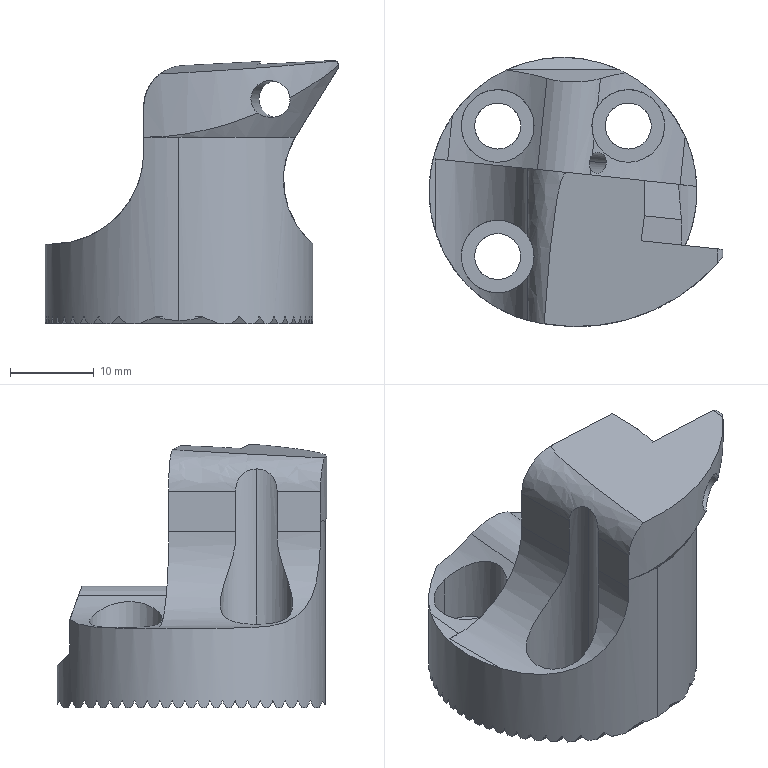CAM job | Mastercam | 3-axis milling, 5-axis milling, drilling
Tools:
tool_number,name,type,diameter_mm,corner_radius_mm,flutes,flute_length_mm,overall_length_mm,shoulder_length_mm,holder_diameter_mm,length_offset,diameter_offset,default_rpm,default_feed_mm_min,default_plunge_mm_min,coolant
1,8 Flat End Mill,end mill,8,0,4,35,35,35,50,1,1,1250,150,600,COOL_OFF
2,12 Flat End Mill Rough,end mill,12,0,4,25,25,25,50,2,2,833,99.96,600,COOL_OFF
2,2.5 Drill,drill,2.5,0,2,40,40,40,50,2,2,2400,288,600,COOL_OFF
3,10 Spot Drill,drill,10,0,2,25,30,30,50,3,3,600,72,600,COOL_OFF
4,12 Flat End Mill Rough,end mill,12,0,4,35,35,35,50,4,4,833,99.96,600,COOL_OFF
4,11 Carbide Drill,drill,11,0,2,25,40,40,50,4,4,545,65.4,600,COOL_OFF
5,4 Flat End Mill Rough,end mill,4,0,4,20,20,20,31.877,5,5,2500,300,600,COOL_OFF
5,8 Flat End Mill Rough,end mill,8,0,4,25,25,25,50,5,5,1250,150,600,COOL_OFF
6,3 Flat End Mill Rough,end mill,3,0,4,20,20,20,31.877,6,6,3333,399.96,600,COOL_OFF
6,8 Flat End Mill Finish,end mill,8,0,4,25,25,25,50,6,6,1250,150,600,COOL_OFF
7,6 Carbide Chamfer Mill,chamfer mill,6,0,4,25,25,25,50,7,7,4166,499.92,600,COOL_OFF
7,3 Flat End Mill Finish,end mill,3,0,4,20,20,20,31.877,7,7,3333,399.96,600,COOL_OFF
8,2 x 7deg Chamfer Mill,chamfer mill,6,0,4,17,20,20,50,8,8,4167,500.04,600,COOL_OFF
8,25 60deg Thread cutter,thread mill,25,0,4,10,50,10,50,8,8,2000,240,600,COOL_OFF
9,12 Flat End Mill Finish,end mill,12,0,4,30,35,30,42.012,9,9,833,99.96,600,COOL_OFF
9,8.7 Carbide Drill,drill,8.7,0,2,25,50,40,50,9,9,690,82.8,600,COOL_OFF
10,30 Bull Nose Mill,bull end mill,30,0.8,4,25,25,25,50,10,10,400,48,600,COOL_OFF
10,50 Facing,end mill,50,0,4,5,50,18,50,10,10,5000,700,2000,COOL_OFF
11,5.5 Flat End Mill,end mill,5.5,0,4,20,20,20,50,11,11,1818,218.16,600,COOL_OFF
11,5.5 Carbide Drill,drill,5.5,0,2,25,50,40,50,11,11,1091,130.92,600,COOL_OFF
12,6 Chamfer Mill,chamfer mill,6,0,4,25,25,25,50,12,12,4167,500.04,600,COOL_OFF
12,8.7 Carbide Flat drill,drill,8.7,0,2,25,50,40,50,12,12,690,82.8,600,COOL_OFF
13,4.5 Drill,drill,4.5,0,2,40,40,40,50,13,13,1333,159.96,600,COOL_OFF
14,2.4 Thread Mill,thread mill,2.4,0,4,1.5,20,20,50,14,14,2500,300,600,COOL_OFF
14,3.15 Thread Mill,thread mill,3.15,0,4,2.1,20,20,27.495,14,14,1905,228.6,600,COOL_OFF
15,2.5 Ball Mill,ball end mill,2.5,1.25,4,3,20,3,50,15,15,4800,576,600,COOL_OFF
Operations:
seq,operation,operation_type,tool_number,tool_name,tool_diameter_mm,spindle_rpm,feed_mm_min,plunge_mm_min,retract_mm_min,cycle_time_s,wcs,posted,nc_file
1,Contour (2D) - [WCS: Top] - [Tplane: 4X1-A0],Contour,10,50 Facing,50,1600,700,2000,5000,8.609,Top,yes,1.nc
2,Contour (2D) - [WCS: Top] - [Tplane: 4X1-A0],Contour,2,2.5 Drill,2.5,3500,400,2000,1200,25.327,Top,yes,1.nc
3,Drill/Counterbore - [WCS: Top] - [Tplane: 4X1-A0],Drill,3,10 Spot Drill,10,2000,100,600,1200,9.576,Top,yes,1.nc
4,Drill/Counterbore - [WCS: Top] - [Tplane: 4X1-A0],Drill,4,11 Carbide Drill,11,2000,100,600,1200,5.914,Top,yes,1.nc
5,Drill/Counterbore - [WCS: Top] - [Tplane: 4X1-A0],Drill,11,5.5 Carbide Drill,5.5,2200,60,600,1200,49.642,Top,yes,1.nc
6,Contour (2D chamfer) - [WCS: Top] - [Tplane: 4X1-A0],Contour,7,3 Flat End Mill Finish,3,3500,400,2000,1200,18.114,Top,yes,1.nc
7,Contour (2D chamfer) - [WCS: Top] - [Tplane: 4X1-A0],Contour,7,3 Flat End Mill Finish,3,3500,400,2000,1200,6.498,Top,yes,1.nc
8,Contour (2D) - [WCS: Top] - [Tplane: 4X2-A+90],Contour,8,25 60deg Thread cutter,25,4000,1000,2000,1200,57.317,Top,yes,2.nc
9,Circle Mill - [WCS: Top] - [Tplane: 4X1-A0],CircleMill,5,8 Flat End Mill Rough,8,3500,400,2000,1200,7.314,Top,yes,2.nc
10,Circle Mill - [WCS: Top] - [Tplane: 4X1-A0],CircleMill,6,8 Flat End Mill Finish,8,3500,400,2000,1200,8.519,Top,yes,2.nc
11,Drill/Counterbore - [WCS: Top] - [Tplane: Top],Drill,3,10 Spot Drill,10,2000,100,600,1200,6.854,Top,yes,2.nc
12,Peck Drill - [WCS: Top] - [Tplane: Top],Drill,9,8.7 Carbide Drill,8.7,2000,100,600,1200,66.341,Top,yes,2.nc
13,Drill/Counterbore - [WCS: Top] - [Tplane: Top],Drill,12,8.7 Carbide Flat drill,8.7,2000,100,600,1200,10.69,Top,yes,2.nc
14,2D High Speed (2D Dynamic Mill) - [WCS: Top] - [Tplane: Ins],HighSpeed2D,4,11 Carbide Drill,11,3500,2500,600,1200,130.359,Top,yes,3.nc
15,Contour (2D) - [WCS: Top] - [Tplane: Out],Contour,1,8 Flat End Mill,8,3500,600,2000,1200,12.412,Top,yes,3.nc
16,Peck Drill - [WCS: Top] - [Tplane: Out],Drill,2,2.5 Drill,2.5,1500,15,600,1200,42.705,Top,yes,3.nc
17,2D High Speed (2D Dynamic Mill) - [WCS: Top] - [Tplane: Ins],HighSpeed2D,4,11 Carbide Drill,11,3500,2500,600,1200,20.916,Top,yes,3.nc
18,Contour (2D) - [WCS: Top] - [Tplane: Ins],Contour,4,11 Carbide Drill,11,3500,1500,2000,1200,7.258,Top,yes,3.nc
19,Contour (Ramp) - [WCS: Top] - [Tplane: 0d],Contour,4,11 Carbide Drill,11,3500,1500,2000,1200,3.059,Top,yes,3.nc
20,Contour (2D) - [WCS: Top] - [Tplane: 0d],Contour,4,11 Carbide Drill,11,3500,1000,2000,1200,19.893,Top,yes,3.nc
21,Stock model - [WCS: Top] - [Tplane: Top] - 1,139,,,,0,0,0,0,0,Top,no,
22,2D High Speed (2D Dynamic Mill) - [WCS: Top] - [Tplane: Ins-1],HighSpeed2D,4,11 Carbide Drill,11,3500,2500,600,1200,103.475,Top,yes,3.nc
23,Contour (Ramp) - [WCS: Top] - [Tplane: 45d],Contour,4,11 Carbide Drill,11,3500,1500,2000,1200,2.918,Top,yes,3.nc
24,Contour (2D) - [WCS: Top] - [Tplane: Ins],Contour,5,8 Flat End Mill Rough,8,4000,600,2000,1200,388.29,Top,yes,3.nc
25,Contour (Remachining) - [WCS: Top] - [Tplane: Ins],Contour,6,8 Flat End Mill Finish,8,4500,400,2000,1200,117.447,Top,yes,3.nc
26,Contour (2D) - [WCS: Top] - [Tplane: Ins],Contour,7,3 Flat End Mill Finish,3,4500,400,2000,1200,23.529,Top,yes,3.nc
27,Contour (2D) - [WCS: Top] - [Tplane: Ins],Contour,7,3 Flat End Mill Finish,3,4500,400,2000,1200,23.53,Top,yes,3.nc
28,Contour (2D chamfer) - [WCS: Top] - [Tplane: Ins],Contour,8,25 60deg Thread cutter,25,4000,400,2000,1200,17.385,Top,yes,3.nc
29,Contour (2D) - [WCS: Top] - [Tplane: Ins],Contour,9,8.7 Carbide Drill,8.7,3500,600,2000,1200,5.303,Top,yes,3.nc
30,Contour (2D) - [WCS: Top] - [Tplane: 0d],Contour,9,8.7 Carbide Drill,8.7,3500,600,2000,1200,3.458,Top,yes,3.nc
31,Contour (2D) - [WCS: Top] - [Tplane: 0d],Contour,9,8.7 Carbide Drill,8.7,3500,600,2000,1200,8.749,Top,yes,3.nc
32,Contour (2D) - [WCS: Top] - [Tplane: Ins-1],Contour,9,8.7 Carbide Drill,8.7,3500,600,2000,1200,5.914,Top,yes,3.nc
33,Contour (2D) - [WCS: Top] - [Tplane: 45d],Contour,9,8.7 Carbide Drill,8.7,3500,600,2000,1200,3.319,Top,yes,3.nc
34,Contour (2D) - [WCS: Top] - [Tplane: Ins],Contour,10,50 Facing,50,3500,600,2000,1200,6.703,Top,yes,3.nc
35,Drill/Counterbore - [WCS: Top] - [Tplane: Ins],Drill,12,8.7 Carbide Flat drill,8.7,2000,100,600,1200,2.403,Top,yes,3.nc
36,Peck Drill - [WCS: Top] - [Tplane: Ins],Drill,13,4.5 Drill,4.5,1000,60,600,1200,11.807,Top,yes,3.nc
37,Drill/Counterbore - [WCS: Top] - [Tplane: CB],Drill,11,5.5 Carbide Drill,5.5,2500,100,600,1200,3.129,Top,yes,3.nc
38,Thread Mill - [WCS: Top] - [Tplane: Ins],ThreadMill,14,3.15 Thread Mill,3.15,3000,300,2000,1200,50.978,Top,yes,3.nc
39,Deburr 5-axis - [WCS: Top] - [Tplane: Top],459,15,2.5 Ball Mill,2.5,4800,600,2000,1200,12.744,Top,yes,3.nc
40,Deburr 5-axis - [WCS: Top] - [Tplane: Top],459,15,2.5 Ball Mill,2.5,4800,600,2000,1200,6.635,Top,yes,3.nc